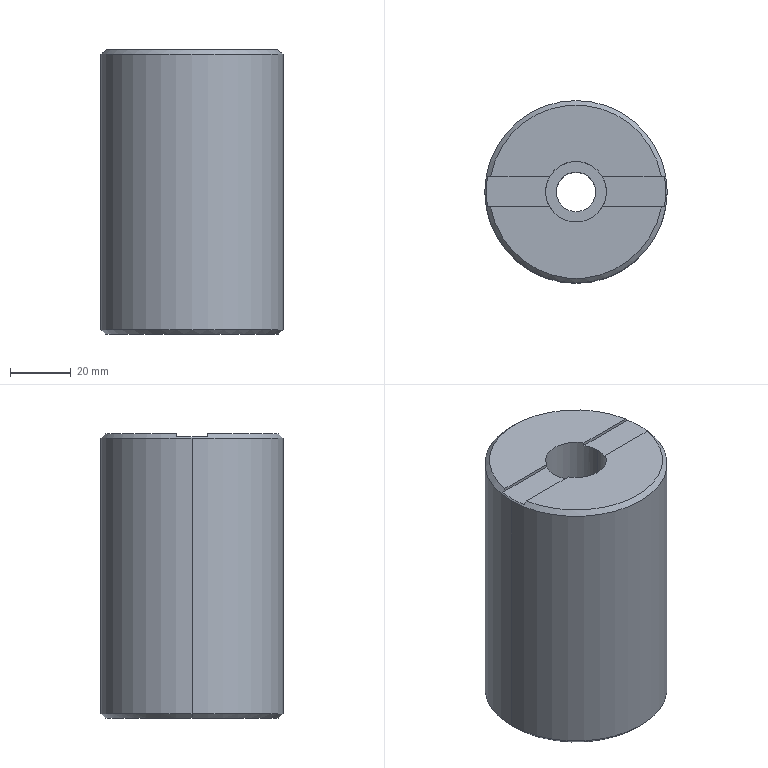Part | 1 solid | 20 faces | box 60 x 60 x 93.5 mm | volume 246072 mm3 | plane 10 | cylinder 6 | cone 4 | commonest cylinder face diameters 13 x2 20 x2 60 x2